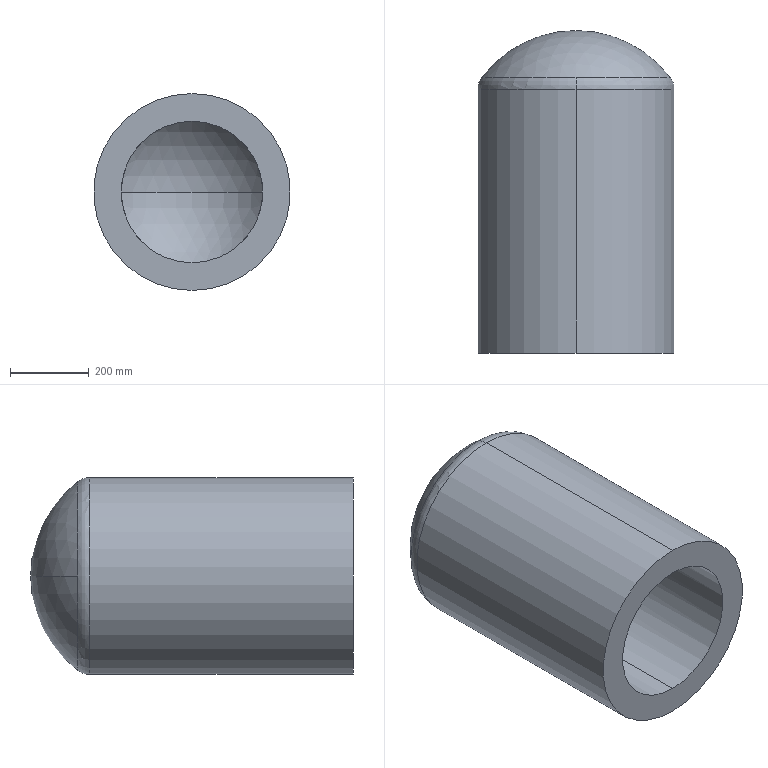Part | SolidWorks | features Fillet 1, Revolution 1, Shell 1 | 1 solid | 11 faces | box 500 x 820 x 500 mm | volume 76793679 mm3 | sphere 4 | cylinder 4 | torus 2 | plane 1 | commonest cylinder face diameters 360 x2 500 x2
STEP:
#1=CARTESIAN_POINT('',(0.,750.,0.));
#2=VERTEX_POINT('',#1);
#3=CARTESIAN_POINT('',(180.,663.178,0.));
#4=VERTEX_POINT('',#3);
#5=CARTESIAN_POINT('',(0.,520.,0.));
#6=DIRECTION('',(0.,0.,-1.));
#7=DIRECTION('',(-1.,0.,0.));
#8=AXIS2_PLACEMENT_3D('',#5,#6,#7);
#9=CIRCLE('',#8,230.);
#10=EDGE_CURVE('',#2,#4,#9,.T.);
#11=ORIENTED_EDGE('',*,*,#10,.F.);
#12=CARTESIAN_POINT('',(-180.,663.178,0.));
#13=VERTEX_POINT('',#12);
#14=CARTESIAN_POINT('',(0.,520.,0.));
#15=DIRECTION('',(0.,0.,1.));
#16=DIRECTION('',(1.,0.,0.));
#17=AXIS2_PLACEMENT_3D('',#14,#15,#16);
#18=CIRCLE('',#17,230.);
#19=EDGE_CURVE('',#2,#13,#18,.T.);
#20=ORIENTED_EDGE('',*,*,#19,.T.);
#21=CARTESIAN_POINT('',(0.,663.178,-180.));
#22=VERTEX_POINT('',#21);
#23=CARTESIAN_POINT('',(0.,663.178,0.));
#24=DIRECTION('',(0.,-1.,0.));
#25=DIRECTION('',(0.,0.,-1.));
#26=AXIS2_PLACEMENT_3D('',#23,#24,#25);
#27=CIRCLE('',#26,180.);
#28=EDGE_CURVE('',#13,#22,#27,.T.);
#29=ORIENTED_EDGE('',*,*,#28,.T.);
#30=CARTESIAN_POINT('',(0.,663.178,0.));
#31=DIRECTION('',(0.,-1.,0.));
#32=DIRECTION('',(0.,0.,-1.));
#33=AXIS2_PLACEMENT_3D('',#30,#31,#32);
#34=CIRCLE('',#33,180.);
#35=EDGE_CURVE('',#22,#4,#34,.T.);
#36=ORIENTED_EDGE('',*,*,#35,.T.);
#37=EDGE_LOOP('',(#11,#20,#29,#36));
#38=FACE_OUTER_BOUND('',#37,.T.);
#39=CARTESIAN_POINT('',(0.,520.,0.));
#40=DIRECTION('',(0.,0.,1.));
#41=DIRECTION('',(1.,0.,0.));
#42=AXIS2_PLACEMENT_3D('',#39,#40,#41);
#43=SPHERICAL_SURFACE('',#42,230.);
#44=ADVANCED_FACE('',(#38),#43,.F.);
#45=CARTESIAN_POINT('',(0.,663.178,180.));
#46=VERTEX_POINT('',#45);
#47=CARTESIAN_POINT('',(0.,663.178,0.));
#48=DIRECTION('',(0.,-1.,0.));
#49=DIRECTION('',(0.,0.,-1.));
#50=AXIS2_PLACEMENT_3D('',#47,#48,#49);
#51=CIRCLE('',#50,180.);
#52=EDGE_CURVE('',#46,#13,#51,.T.);
#53=ORIENTED_EDGE('',*,*,#52,.F.);
#54=CARTESIAN_POINT('',(0.,0.,180.));
#55=VERTEX_POINT('',#54);
#56=CARTESIAN_POINT('',(0.,0.,180.));
#57=DIRECTION('',(0.,-1.,0.));
#58=VECTOR('',#57,1000.);
#59=LINE('',#56,#58);
#60=EDGE_CURVE('',#46,#55,#59,.T.);
#61=ORIENTED_EDGE('',*,*,#60,.T.);
#62=CARTESIAN_POINT('',(0.,0.,-180.));
#63=VERTEX_POINT('',#62);
#64=CARTESIAN_POINT('',(0.,0.,0.));
#65=DIRECTION('',(0.,-1.,0.));
#66=DIRECTION('',(0.,0.,-1.));
#67=AXIS2_PLACEMENT_3D('',#64,#65,#66);
#68=CIRCLE('',#67,180.);
#69=EDGE_CURVE('',#55,#63,#68,.T.);
#70=ORIENTED_EDGE('',*,*,#69,.T.);
#71=CARTESIAN_POINT('',(0.,0.,-180.));
#72=DIRECTION('',(0.,-1.,0.));
#73=VECTOR('',#72,1000.);
#74=LINE('',#71,#73);
#75=EDGE_CURVE('',#22,#63,#74,.T.);
#76=ORIENTED_EDGE('',*,*,#75,.F.);
#77=ORIENTED_EDGE('',*,*,#28,.F.);
#78=EDGE_LOOP('',(#53,#61,#70,#76,#77));
#79=FACE_OUTER_BOUND('',#78,.T.);
#80=CARTESIAN_POINT('',(0.,0.,0.));
#81=DIRECTION('',(0.,-1.,0.));
#82=DIRECTION('',(0.,0.,-1.));
#83=AXIS2_PLACEMENT_3D('',#80,#81,#82);
#84=CYLINDRICAL_SURFACE('',#83,180.);
#85=ADVANCED_FACE('',(#79),#84,.F.);
#86=CARTESIAN_POINT('',(0.,700.,240.));
#87=VERTEX_POINT('',#86);
#88=CARTESIAN_POINT('',(240.,700.,0.));
#89=VERTEX_POINT('',#88);
#90=CARTESIAN_POINT('',(0.,700.,0.));
#91=DIRECTION('',(0.,1.,0.));
#92=DIRECTION('',(0.,0.,-1.));
#93=AXIS2_PLACEMENT_3D('',#90,#91,#92);
#94=CIRCLE('',#93,240.);
#95=EDGE_CURVE('',#87,#89,#94,.T.);
#96=ORIENTED_EDGE('',*,*,#95,.F.);
#97=CARTESIAN_POINT('',(0.,670.,250.));
#98=VERTEX_POINT('',#97);
#99=CARTESIAN_POINT('',(0.,670.,200.));
#100=DIRECTION('',(1.,0.,0.));
#101=DIRECTION('',(0.,0.,-1.));
#102=AXIS2_PLACEMENT_3D('',#99,#100,#101);
#103=CIRCLE('',#102,50.);
#104=EDGE_CURVE('',#87,#98,#103,.T.);
#105=ORIENTED_EDGE('',*,*,#104,.T.);
#106=CARTESIAN_POINT('',(0.,670.,-250.));
#107=VERTEX_POINT('',#106);
#108=CARTESIAN_POINT('',(0.,670.,0.));
#109=DIRECTION('',(0.,-1.,0.));
#110=DIRECTION('',(0.,0.,-1.));
#111=AXIS2_PLACEMENT_3D('',#108,#109,#110);
#112=CIRCLE('',#111,250.);
#113=EDGE_CURVE('',#107,#98,#112,.T.);
#114=ORIENTED_EDGE('',*,*,#113,.F.);
#115=CARTESIAN_POINT('',(0.,700.,-240.));
#116=VERTEX_POINT('',#115);
#117=CARTESIAN_POINT('',(0.,670.,-200.));
#118=DIRECTION('',(-1.,0.,0.));
#119=DIRECTION('',(0.,0.,1.));
#120=AXIS2_PLACEMENT_3D('',#117,#118,#119);
#121=CIRCLE('',#120,50.);
#122=EDGE_CURVE('',#116,#107,#121,.T.);
#123=ORIENTED_EDGE('',*,*,#122,.F.);
#124=CARTESIAN_POINT('',(0.,700.,0.));
#125=DIRECTION('',(0.,1.,0.));
#126=DIRECTION('',(0.,0.,-1.));
#127=AXIS2_PLACEMENT_3D('',#124,#125,#126);
#128=CIRCLE('',#127,240.);
#129=EDGE_CURVE('',#89,#116,#128,.T.);
#130=ORIENTED_EDGE('',*,*,#129,.F.);
#131=EDGE_LOOP('',(#96,#105,#114,#123,#130));
#132=FACE_OUTER_BOUND('',#131,.T.);
#133=CARTESIAN_POINT('',(0.,670.,0.));
#134=DIRECTION('',(0.,-1.,0.));
#135=DIRECTION('',(0.,0.,-1.));
#136=AXIS2_PLACEMENT_3D('',#133,#134,#135);
#137=TOROIDAL_SURFACE('',#136,200.,50.);
#138=ADVANCED_FACE('',(#132),#137,.T.);
#139=CARTESIAN_POINT('',(0.,820.,0.));
#140=VERTEX_POINT('',#139);
#141=CARTESIAN_POINT('',(0.,520.,0.));
#142=DIRECTION('',(0.,0.,-1.));
#143=DIRECTION('',(-1.,0.,0.));
#144=AXIS2_PLACEMENT_3D('',#141,#142,#143);
#145=CIRCLE('',#144,300.);
#146=EDGE_CURVE('',#140,#89,#145,.T.);
#147=ORIENTED_EDGE('',*,*,#146,.F.);
#148=CARTESIAN_POINT('',(-240.,700.,0.));
#149=VERTEX_POINT('',#148);
#150=CARTESIAN_POINT('',(0.,520.,0.));
#151=DIRECTION('',(0.,0.,1.));
#152=DIRECTION('',(1.,0.,0.));
#153=AXIS2_PLACEMENT_3D('',#150,#151,#152);
#154=CIRCLE('',#153,300.);
#155=EDGE_CURVE('',#140,#149,#154,.T.);
#156=ORIENTED_EDGE('',*,*,#155,.T.);
#157=CARTESIAN_POINT('',(0.,700.,0.));
#158=DIRECTION('',(0.,1.,0.));
#159=DIRECTION('',(0.,0.,-1.));
#160=AXIS2_PLACEMENT_3D('',#157,#158,#159);
#161=CIRCLE('',#160,240.);
#162=EDGE_CURVE('',#149,#87,#161,.T.);
#163=ORIENTED_EDGE('',*,*,#162,.T.);
#164=ORIENTED_EDGE('',*,*,#95,.T.);
#165=EDGE_LOOP('',(#147,#156,#163,#164));
#166=FACE_OUTER_BOUND('',#165,.T.);
#167=CARTESIAN_POINT('',(0.,520.,0.));
#168=DIRECTION('',(0.,0.,1.));
#169=DIRECTION('',(1.,0.,0.));
#170=AXIS2_PLACEMENT_3D('',#167,#168,#169);
#171=SPHERICAL_SURFACE('',#170,300.);
#172=ADVANCED_FACE('',(#166),#171,.T.);
#173=ORIENTED_EDGE('',*,*,#113,.T.);
#174=CARTESIAN_POINT('',(0.,0.,250.));
#175=VERTEX_POINT('',#174);
#176=CARTESIAN_POINT('',(0.,0.,250.));
#177=DIRECTION('',(0.,-1.,0.));
#178=VECTOR('',#177,1000.);
#179=LINE('',#176,#178);
#180=EDGE_CURVE('',#98,#175,#179,.T.);
#181=ORIENTED_EDGE('',*,*,#180,.T.);
#182=CARTESIAN_POINT('',(0.,0.,-250.));
#183=VERTEX_POINT('',#182);
#184=CARTESIAN_POINT('',(0.,0.,0.));
#185=DIRECTION('',(0.,-1.,0.));
#186=DIRECTION('',(0.,0.,-1.));
#187=AXIS2_PLACEMENT_3D('',#184,#185,#186);
#188=CIRCLE('',#187,250.);
#189=EDGE_CURVE('',#183,#175,#188,.T.);
#190=ORIENTED_EDGE('',*,*,#189,.F.);
#191=CARTESIAN_POINT('',(0.,0.,-250.));
#192=DIRECTION('',(0.,-1.,0.));
#193=VECTOR('',#192,1000.);
#194=LINE('',#191,#193);
#195=EDGE_CURVE('',#107,#183,#194,.T.);
#196=ORIENTED_EDGE('',*,*,#195,.F.);
#197=EDGE_LOOP('',(#173,#181,#190,#196));
#198=FACE_OUTER_BOUND('',#197,.T.);
#199=CARTESIAN_POINT('',(0.,0.,0.));
#200=DIRECTION('',(0.,-1.,0.));
#201=DIRECTION('',(0.,0.,-1.));
#202=AXIS2_PLACEMENT_3D('',#199,#200,#201);
#203=CYLINDRICAL_SURFACE('',#202,250.);
#204=ADVANCED_FACE('',(#198),#203,.T.);
#205=CARTESIAN_POINT('',(0.,0.,0.));
#206=DIRECTION('',(0.,-1.,0.));
#207=DIRECTION('',(0.,0.,-1.));
#208=AXIS2_PLACEMENT_3D('',#205,#206,#207);
#209=CIRCLE('',#208,180.);
#210=EDGE_CURVE('',#63,#55,#209,.T.);
#211=ORIENTED_EDGE('',*,*,#210,.F.);
#212=ORIENTED_EDGE('',*,*,#69,.F.);
#213=EDGE_LOOP('',(#211,#212));
#214=FACE_BOUND('',#213,.T.);
#215=ORIENTED_EDGE('',*,*,#189,.T.);
#216=CARTESIAN_POINT('',(0.,0.,0.));
#217=DIRECTION('',(0.,-1.,0.));
#218=DIRECTION('',(0.,0.,-1.));
#219=AXIS2_PLACEMENT_3D('',#216,#217,#218);
#220=CIRCLE('',#219,250.);
#221=EDGE_CURVE('',#175,#183,#220,.T.);
#222=ORIENTED_EDGE('',*,*,#221,.T.);
#223=EDGE_LOOP('',(#215,#222));
#224=FACE_OUTER_BOUND('',#223,.T.);
#225=CARTESIAN_POINT('',(250.,0.,0.));
#226=DIRECTION('',(0.,-1.,0.));
#227=DIRECTION('',(0.,0.,-1.));
#228=AXIS2_PLACEMENT_3D('',#225,#226,#227);
#229=PLANE('',#228);
#230=ADVANCED_FACE('',(#214,#224),#229,.T.);
#231=ORIENTED_EDGE('',*,*,#180,.F.);
#232=CARTESIAN_POINT('',(0.,670.,0.));
#233=DIRECTION('',(0.,-1.,0.));
#234=DIRECTION('',(0.,0.,-1.));
#235=AXIS2_PLACEMENT_3D('',#232,#233,#234);
#236=CIRCLE('',#235,250.);
#237=EDGE_CURVE('',#98,#107,#236,.T.);
#238=ORIENTED_EDGE('',*,*,#237,.T.);
#239=ORIENTED_EDGE('',*,*,#195,.T.);
#240=ORIENTED_EDGE('',*,*,#221,.F.);
#241=EDGE_LOOP('',(#231,#238,#239,#240));
#242=FACE_OUTER_BOUND('',#241,.T.);
#243=CARTESIAN_POINT('',(0.,0.,0.));
#244=DIRECTION('',(0.,-1.,0.));
#245=DIRECTION('',(0.,0.,-1.));
#246=AXIS2_PLACEMENT_3D('',#243,#244,#245);
#247=CYLINDRICAL_SURFACE('',#246,250.);
#248=ADVANCED_FACE('',(#242),#247,.T.);
#249=ORIENTED_EDGE('',*,*,#155,.F.);
#250=ORIENTED_EDGE('',*,*,#146,.T.);
#251=ORIENTED_EDGE('',*,*,#129,.T.);
#252=CARTESIAN_POINT('',(0.,700.,0.));
#253=DIRECTION('',(0.,1.,0.));
#254=DIRECTION('',(0.,0.,-1.));
#255=AXIS2_PLACEMENT_3D('',#252,#253,#254);
#256=CIRCLE('',#255,240.);
#257=EDGE_CURVE('',#116,#149,#256,.T.);
#258=ORIENTED_EDGE('',*,*,#257,.T.);
#259=EDGE_LOOP('',(#249,#250,#251,#258));
#260=FACE_OUTER_BOUND('',#259,.T.);
#261=CARTESIAN_POINT('',(0.,520.,0.));
#262=DIRECTION('',(0.,0.,1.));
#263=DIRECTION('',(1.,0.,0.));
#264=AXIS2_PLACEMENT_3D('',#261,#262,#263);
#265=SPHERICAL_SURFACE('',#264,300.);
#266=ADVANCED_FACE('',(#260),#265,.T.);
#267=ORIENTED_EDGE('',*,*,#104,.F.);
#268=ORIENTED_EDGE('',*,*,#162,.F.);
#269=ORIENTED_EDGE('',*,*,#257,.F.);
#270=ORIENTED_EDGE('',*,*,#122,.T.);
#271=ORIENTED_EDGE('',*,*,#237,.F.);
#272=EDGE_LOOP('',(#267,#268,#269,#270,#271));
#273=FACE_OUTER_BOUND('',#272,.T.);
#274=CARTESIAN_POINT('',(0.,670.,0.));
#275=DIRECTION('',(0.,-1.,0.));
#276=DIRECTION('',(0.,0.,-1.));
#277=AXIS2_PLACEMENT_3D('',#274,#275,#276);
#278=TOROIDAL_SURFACE('',#277,200.,50.);
#279=ADVANCED_FACE('',(#273),#278,.T.);
#280=ORIENTED_EDGE('',*,*,#60,.F.);
#281=CARTESIAN_POINT('',(0.,663.178,0.));
#282=DIRECTION('',(0.,-1.,0.));
#283=DIRECTION('',(0.,0.,-1.));
#284=AXIS2_PLACEMENT_3D('',#281,#282,#283);
#285=CIRCLE('',#284,180.);
#286=EDGE_CURVE('',#4,#46,#285,.T.);
#287=ORIENTED_EDGE('',*,*,#286,.F.);
#288=ORIENTED_EDGE('',*,*,#35,.F.);
#289=ORIENTED_EDGE('',*,*,#75,.T.);
#290=ORIENTED_EDGE('',*,*,#210,.T.);
#291=EDGE_LOOP('',(#280,#287,#288,#289,#290));
#292=FACE_OUTER_BOUND('',#291,.T.);
#293=CARTESIAN_POINT('',(0.,0.,0.));
#294=DIRECTION('',(0.,-1.,0.));
#295=DIRECTION('',(0.,0.,-1.));
#296=AXIS2_PLACEMENT_3D('',#293,#294,#295);
#297=CYLINDRICAL_SURFACE('',#296,180.);
#298=ADVANCED_FACE('',(#292),#297,.F.);
#299=ORIENTED_EDGE('',*,*,#19,.F.);
#300=ORIENTED_EDGE('',*,*,#10,.T.);
#301=ORIENTED_EDGE('',*,*,#286,.T.);
#302=ORIENTED_EDGE('',*,*,#52,.T.);
#303=EDGE_LOOP('',(#299,#300,#301,#302));
#304=FACE_OUTER_BOUND('',#303,.T.);
#305=CARTESIAN_POINT('',(0.,520.,0.));
#306=DIRECTION('',(0.,0.,1.));
#307=DIRECTION('',(1.,0.,0.));
#308=AXIS2_PLACEMENT_3D('',#305,#306,#307);
#309=SPHERICAL_SURFACE('',#308,230.);
#310=ADVANCED_FACE('',(#304),#309,.F.);
#311=CLOSED_SHELL('',(#44,#85,#138,#172,#204,#230,#248,#266,#279,#298,#310));
#312=MANIFOLD_SOLID_BREP('',#311);
#313=CARTESIAN_POINT('',(0.,0.,0.));
#314=DIRECTION('',(0.,0.,1.));
#315=DIRECTION('',(1.,0.,0.));
#316=AXIS2_PLACEMENT_3D('',#313,#314,#315);
#317=(LENGTH_UNIT()NAMED_UNIT(*)SI_UNIT(.MILLI.,.METRE.));
#318=UNCERTAINTY_MEASURE_WITH_UNIT(LENGTH_MEASURE(0.00001),#317,'','');
#319=(NAMED_UNIT(*)PLANE_ANGLE_UNIT()SI_UNIT($,.RADIAN.));
#320=(NAMED_UNIT(*)SI_UNIT($,.STERADIAN.)SOLID_ANGLE_UNIT());
#321=(GEOMETRIC_REPRESENTATION_CONTEXT(3)GLOBAL_UNCERTAINTY_ASSIGNED_CONTEXT((#318))GLOBAL_UNIT_ASSIGNED_CONTEXT((#317,#319,#320))REPRESENTATION_CONTEXT('',''));
#322=ADVANCED_BREP_SHAPE_REPRESENTATION('',(#312,#316),#321);